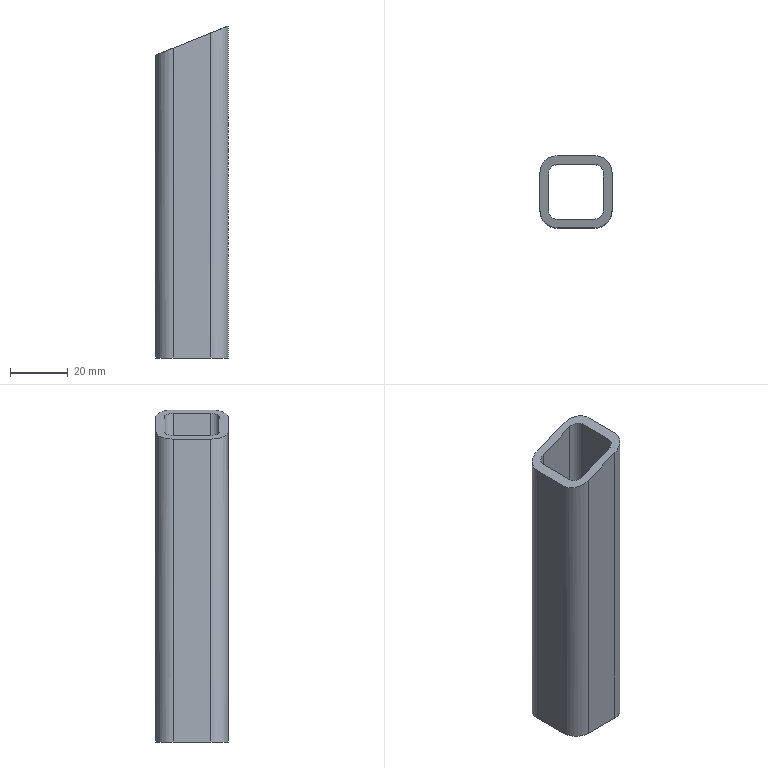Part | STEP file | ISO 10799-2 25x25x3 1784907954146 | 1 solid | 18 faces | box 25 x 25 x 115.036 mm | volume 26491 mm3 | plane 10 | cylinder 8 | commonest cylinder face diameters 6 x4 12 x4
STEP:
#1=CARTESIAN_POINT('',(12.5,6.5,115.036));
#2=VERTEX_POINT('',#1);
#3=CARTESIAN_POINT('',(12.5,-6.5,115.036));
#4=VERTEX_POINT('',#3);
#5=CARTESIAN_POINT('',(12.5,3.25,115.036));
#6=DIRECTION('',(0.,-1.,0.));
#7=VECTOR('',#6,10.);
#8=LINE('',#5,#7);
#9=EDGE_CURVE('',#2,#4,#8,.T.);
#10=ORIENTED_EDGE('',*,*,#9,.F.);
#11=CARTESIAN_POINT('',(6.5,12.5,112.619));
#12=VERTEX_POINT('',#11);
#13=CARTESIAN_POINT('',(6.5,6.5,112.619));
#14=DIRECTION('',(0.3737,0.,-0.9275));
#15=DIRECTION('',(-0.9275,0.,-0.3737));
#16=AXIS2_PLACEMENT_3D('',#13,#14,#15);
#17=ELLIPSE('',#16,6.469,6.);
#18=EDGE_CURVE('',#12,#2,#17,.T.);
#19=ORIENTED_EDGE('',*,*,#18,.F.);
#20=CARTESIAN_POINT('',(-6.5,12.5,107.381));
#21=VERTEX_POINT('',#20);
#22=CARTESIAN_POINT('',(-40.927,12.5,93.51));
#23=DIRECTION('',(0.9275,0.,0.3737));
#24=VECTOR('',#23,10.);
#25=LINE('',#22,#24);
#26=EDGE_CURVE('',#21,#12,#25,.T.);
#27=ORIENTED_EDGE('',*,*,#26,.F.);
#28=CARTESIAN_POINT('',(-12.5,6.5,104.964));
#29=VERTEX_POINT('',#28);
#30=CARTESIAN_POINT('',(-6.5,6.5,107.381));
#31=DIRECTION('',(0.3737,0.,-0.9275));
#32=DIRECTION('',(0.9275,0.,0.3737));
#33=AXIS2_PLACEMENT_3D('',#30,#31,#32);
#34=ELLIPSE('',#33,6.469,6.);
#35=EDGE_CURVE('',#29,#21,#34,.T.);
#36=ORIENTED_EDGE('',*,*,#35,.F.);
#37=CARTESIAN_POINT('',(-12.5,-6.5,104.964));
#38=VERTEX_POINT('',#37);
#39=CARTESIAN_POINT('',(-12.5,-3.25,104.964));
#40=DIRECTION('',(0.,1.,0.));
#41=VECTOR('',#40,10.);
#42=LINE('',#39,#41);
#43=EDGE_CURVE('',#38,#29,#42,.T.);
#44=ORIENTED_EDGE('',*,*,#43,.F.);
#45=CARTESIAN_POINT('',(-6.5,-12.5,107.381));
#46=VERTEX_POINT('',#45);
#47=CARTESIAN_POINT('',(-6.5,-6.5,107.381));
#48=DIRECTION('',(0.3737,0.,-0.9275));
#49=DIRECTION('',(0.9275,0.,0.3737));
#50=AXIS2_PLACEMENT_3D('',#47,#48,#49);
#51=ELLIPSE('',#50,6.469,6.);
#52=EDGE_CURVE('',#46,#38,#51,.T.);
#53=ORIENTED_EDGE('',*,*,#52,.F.);
#54=CARTESIAN_POINT('',(6.5,-12.5,112.619));
#55=VERTEX_POINT('',#54);
#56=CARTESIAN_POINT('',(-35.334,-12.5,95.763));
#57=DIRECTION('',(-0.9275,0.,-0.3737));
#58=VECTOR('',#57,10.);
#59=LINE('',#56,#58);
#60=EDGE_CURVE('',#55,#46,#59,.T.);
#61=ORIENTED_EDGE('',*,*,#60,.F.);
#62=CARTESIAN_POINT('',(6.5,-6.5,112.619));
#63=DIRECTION('',(0.3737,0.,-0.9275));
#64=DIRECTION('',(-0.9275,0.,-0.3737));
#65=AXIS2_PLACEMENT_3D('',#62,#63,#64);
#66=ELLIPSE('',#65,6.469,6.);
#67=EDGE_CURVE('',#4,#55,#66,.T.);
#68=ORIENTED_EDGE('',*,*,#67,.F.);
#69=EDGE_LOOP('',(#10,#19,#27,#36,#44,#53,#61,#68));
#70=FACE_OUTER_BOUND('',#69,.T.);
#71=CARTESIAN_POINT('',(-6.5,-9.5,107.381));
#72=VERTEX_POINT('',#71);
#73=CARTESIAN_POINT('',(6.5,-9.5,112.619));
#74=VERTEX_POINT('',#73);
#75=CARTESIAN_POINT('',(-35.334,-9.5,95.763));
#76=DIRECTION('',(0.9275,0.,0.3737));
#77=VECTOR('',#76,10.);
#78=LINE('',#75,#77);
#79=EDGE_CURVE('',#72,#74,#78,.T.);
#80=ORIENTED_EDGE('',*,*,#79,.F.);
#81=CARTESIAN_POINT('',(-9.5,-6.5,106.172));
#82=VERTEX_POINT('',#81);
#83=CARTESIAN_POINT('',(-6.5,-6.5,107.381));
#84=DIRECTION('',(-0.3737,0.,0.9275));
#85=DIRECTION('',(0.9275,0.,0.3737));
#86=AXIS2_PLACEMENT_3D('',#83,#84,#85);
#87=ELLIPSE('',#86,3.234,3.);
#88=EDGE_CURVE('',#82,#72,#87,.T.);
#89=ORIENTED_EDGE('',*,*,#88,.F.);
#90=CARTESIAN_POINT('',(-9.5,6.5,106.172));
#91=VERTEX_POINT('',#90);
#92=CARTESIAN_POINT('',(-9.5,-3.25,106.172));
#93=DIRECTION('',(0.,-1.,0.));
#94=VECTOR('',#93,10.);
#95=LINE('',#92,#94);
#96=EDGE_CURVE('',#91,#82,#95,.T.);
#97=ORIENTED_EDGE('',*,*,#96,.F.);
#98=CARTESIAN_POINT('',(-6.5,9.5,107.381));
#99=VERTEX_POINT('',#98);
#100=CARTESIAN_POINT('',(-6.5,6.5,107.381));
#101=DIRECTION('',(-0.3737,0.,0.9275));
#102=DIRECTION('',(0.9275,0.,0.3737));
#103=AXIS2_PLACEMENT_3D('',#100,#101,#102);
#104=ELLIPSE('',#103,3.234,3.);
#105=EDGE_CURVE('',#99,#91,#104,.T.);
#106=ORIENTED_EDGE('',*,*,#105,.F.);
#107=CARTESIAN_POINT('',(6.5,9.5,112.619));
#108=VERTEX_POINT('',#107);
#109=CARTESIAN_POINT('',(-40.927,9.5,93.51));
#110=DIRECTION('',(-0.9275,0.,-0.3737));
#111=VECTOR('',#110,10.);
#112=LINE('',#109,#111);
#113=EDGE_CURVE('',#108,#99,#112,.T.);
#114=ORIENTED_EDGE('',*,*,#113,.F.);
#115=CARTESIAN_POINT('',(9.5,6.5,113.828));
#116=VERTEX_POINT('',#115);
#117=CARTESIAN_POINT('',(6.5,6.5,112.619));
#118=DIRECTION('',(-0.3737,0.,0.9275));
#119=DIRECTION('',(-0.9275,0.,-0.3737));
#120=AXIS2_PLACEMENT_3D('',#117,#118,#119);
#121=ELLIPSE('',#120,3.234,3.);
#122=EDGE_CURVE('',#116,#108,#121,.T.);
#123=ORIENTED_EDGE('',*,*,#122,.F.);
#124=CARTESIAN_POINT('',(9.5,-6.5,113.828));
#125=VERTEX_POINT('',#124);
#126=CARTESIAN_POINT('',(9.5,3.25,113.828));
#127=DIRECTION('',(0.,1.,0.));
#128=VECTOR('',#127,10.);
#129=LINE('',#126,#128);
#130=EDGE_CURVE('',#125,#116,#129,.T.);
#131=ORIENTED_EDGE('',*,*,#130,.F.);
#132=CARTESIAN_POINT('',(6.5,-6.5,112.619));
#133=DIRECTION('',(-0.3737,0.,0.9275));
#134=DIRECTION('',(-0.9275,0.,-0.3737));
#135=AXIS2_PLACEMENT_3D('',#132,#133,#134);
#136=ELLIPSE('',#135,3.234,3.);
#137=EDGE_CURVE('',#74,#125,#136,.T.);
#138=ORIENTED_EDGE('',*,*,#137,.F.);
#139=EDGE_LOOP('',(#80,#89,#97,#106,#114,#123,#131,#138));
#140=FACE_BOUND('',#139,.T.);
#141=CARTESIAN_POINT('',(-38.131,0.,94.637));
#142=DIRECTION('',(0.3737,0.,-0.9275));
#143=DIRECTION('',(-0.9275,0.,-0.3737));
#144=AXIS2_PLACEMENT_3D('',#141,#142,#143);
#145=PLANE('',#144);
#146=ADVANCED_FACE('',(#70,#140),#145,.F.);
#147=ORIENTED_EDGE('',*,*,#113,.T.);
#148=CARTESIAN_POINT('',(-6.5,9.5,0.));
#149=VERTEX_POINT('',#148);
#150=CARTESIAN_POINT('',(-6.5,9.5,0.));
#151=DIRECTION('',(0.,0.,1.));
#152=VECTOR('',#151,10.);
#153=LINE('',#150,#152);
#154=EDGE_CURVE('',#149,#99,#153,.T.);
#155=ORIENTED_EDGE('',*,*,#154,.F.);
#156=CARTESIAN_POINT('',(6.5,9.5,0.));
#157=VERTEX_POINT('',#156);
#158=CARTESIAN_POINT('',(-3.25,9.5,0.));
#159=DIRECTION('',(-1.,0.,0.));
#160=VECTOR('',#159,10.);
#161=LINE('',#158,#160);
#162=EDGE_CURVE('',#157,#149,#161,.T.);
#163=ORIENTED_EDGE('',*,*,#162,.F.);
#164=CARTESIAN_POINT('',(6.5,9.5,0.));
#165=DIRECTION('',(0.,0.,1.));
#166=VECTOR('',#165,10.);
#167=LINE('',#164,#166);
#168=EDGE_CURVE('',#157,#108,#167,.T.);
#169=ORIENTED_EDGE('',*,*,#168,.T.);
#170=EDGE_LOOP('',(#147,#155,#163,#169));
#171=FACE_OUTER_BOUND('',#170,.T.);
#172=CARTESIAN_POINT('',(-6.5,9.5,0.));
#173=DIRECTION('',(0.,1.,0.));
#174=DIRECTION('',(0.,0.,1.));
#175=AXIS2_PLACEMENT_3D('',#172,#173,#174);
#176=PLANE('',#175);
#177=ADVANCED_FACE('',(#171),#176,.F.);
#178=ORIENTED_EDGE('',*,*,#105,.T.);
#179=CARTESIAN_POINT('',(-9.5,6.5,0.));
#180=VERTEX_POINT('',#179);
#181=CARTESIAN_POINT('',(-9.5,6.5,0.));
#182=DIRECTION('',(0.,0.,1.));
#183=VECTOR('',#182,10.);
#184=LINE('',#181,#183);
#185=EDGE_CURVE('',#180,#91,#184,.T.);
#186=ORIENTED_EDGE('',*,*,#185,.F.);
#187=CARTESIAN_POINT('',(-6.5,6.5,0.));
#188=DIRECTION('',(0.,0.,1.));
#189=DIRECTION('',(0.,-1.,0.));
#190=AXIS2_PLACEMENT_3D('',#187,#188,#189);
#191=CIRCLE('',#190,3.);
#192=EDGE_CURVE('',#149,#180,#191,.T.);
#193=ORIENTED_EDGE('',*,*,#192,.F.);
#194=ORIENTED_EDGE('',*,*,#154,.T.);
#195=EDGE_LOOP('',(#178,#186,#193,#194));
#196=FACE_OUTER_BOUND('',#195,.T.);
#197=CARTESIAN_POINT('',(-6.5,6.5,0.));
#198=DIRECTION('',(0.,0.,1.));
#199=DIRECTION('',(0.,-1.,0.));
#200=AXIS2_PLACEMENT_3D('',#197,#198,#199);
#201=CYLINDRICAL_SURFACE('',#200,3.);
#202=ADVANCED_FACE('',(#196),#201,.F.);
#203=ORIENTED_EDGE('',*,*,#96,.T.);
#204=CARTESIAN_POINT('',(-9.5,-6.5,0.));
#205=VERTEX_POINT('',#204);
#206=CARTESIAN_POINT('',(-9.5,-6.5,0.));
#207=DIRECTION('',(0.,0.,1.));
#208=VECTOR('',#207,10.);
#209=LINE('',#206,#208);
#210=EDGE_CURVE('',#205,#82,#209,.T.);
#211=ORIENTED_EDGE('',*,*,#210,.F.);
#212=CARTESIAN_POINT('',(-9.5,-3.25,0.));
#213=DIRECTION('',(0.,-1.,0.));
#214=VECTOR('',#213,10.);
#215=LINE('',#212,#214);
#216=EDGE_CURVE('',#180,#205,#215,.T.);
#217=ORIENTED_EDGE('',*,*,#216,.F.);
#218=ORIENTED_EDGE('',*,*,#185,.T.);
#219=EDGE_LOOP('',(#203,#211,#217,#218));
#220=FACE_OUTER_BOUND('',#219,.T.);
#221=CARTESIAN_POINT('',(-9.5,-6.5,0.));
#222=DIRECTION('',(-1.,0.,0.));
#223=DIRECTION('',(0.,0.,1.));
#224=AXIS2_PLACEMENT_3D('',#221,#222,#223);
#225=PLANE('',#224);
#226=ADVANCED_FACE('',(#220),#225,.F.);
#227=ORIENTED_EDGE('',*,*,#88,.T.);
#228=CARTESIAN_POINT('',(-6.5,-9.5,0.));
#229=VERTEX_POINT('',#228);
#230=CARTESIAN_POINT('',(-6.5,-9.5,0.));
#231=DIRECTION('',(0.,0.,1.));
#232=VECTOR('',#231,10.);
#233=LINE('',#230,#232);
#234=EDGE_CURVE('',#229,#72,#233,.T.);
#235=ORIENTED_EDGE('',*,*,#234,.F.);
#236=CARTESIAN_POINT('',(-6.5,-6.5,0.));
#237=DIRECTION('',(0.,0.,1.));
#238=DIRECTION('',(1.,0.,0.));
#239=AXIS2_PLACEMENT_3D('',#236,#237,#238);
#240=CIRCLE('',#239,3.);
#241=EDGE_CURVE('',#205,#229,#240,.T.);
#242=ORIENTED_EDGE('',*,*,#241,.F.);
#243=ORIENTED_EDGE('',*,*,#210,.T.);
#244=EDGE_LOOP('',(#227,#235,#242,#243));
#245=FACE_OUTER_BOUND('',#244,.T.);
#246=CARTESIAN_POINT('',(-6.5,-6.5,0.));
#247=DIRECTION('',(0.,0.,1.));
#248=DIRECTION('',(1.,0.,0.));
#249=AXIS2_PLACEMENT_3D('',#246,#247,#248);
#250=CYLINDRICAL_SURFACE('',#249,3.);
#251=ADVANCED_FACE('',(#245),#250,.F.);
#252=ORIENTED_EDGE('',*,*,#35,.T.);
#253=CARTESIAN_POINT('',(-6.5,12.5,0.));
#254=VERTEX_POINT('',#253);
#255=CARTESIAN_POINT('',(-6.5,12.5,0.));
#256=DIRECTION('',(0.,0.,1.));
#257=VECTOR('',#256,10.);
#258=LINE('',#255,#257);
#259=EDGE_CURVE('',#254,#21,#258,.T.);
#260=ORIENTED_EDGE('',*,*,#259,.F.);
#261=CARTESIAN_POINT('',(-12.5,6.5,0.));
#262=VERTEX_POINT('',#261);
#263=CARTESIAN_POINT('',(-6.5,6.5,0.));
#264=DIRECTION('',(0.,0.,-1.));
#265=DIRECTION('',(0.,-1.,0.));
#266=AXIS2_PLACEMENT_3D('',#263,#264,#265);
#267=CIRCLE('',#266,6.);
#268=EDGE_CURVE('',#262,#254,#267,.T.);
#269=ORIENTED_EDGE('',*,*,#268,.F.);
#270=CARTESIAN_POINT('',(-12.5,6.5,0.));
#271=DIRECTION('',(0.,0.,1.));
#272=VECTOR('',#271,10.);
#273=LINE('',#270,#272);
#274=EDGE_CURVE('',#262,#29,#273,.T.);
#275=ORIENTED_EDGE('',*,*,#274,.T.);
#276=EDGE_LOOP('',(#252,#260,#269,#275));
#277=FACE_OUTER_BOUND('',#276,.T.);
#278=CARTESIAN_POINT('',(-6.5,6.5,0.));
#279=DIRECTION('',(0.,0.,1.));
#280=DIRECTION('',(0.,-1.,0.));
#281=AXIS2_PLACEMENT_3D('',#278,#279,#280);
#282=CYLINDRICAL_SURFACE('',#281,6.);
#283=ADVANCED_FACE('',(#277),#282,.T.);
#284=ORIENTED_EDGE('',*,*,#26,.T.);
#285=CARTESIAN_POINT('',(6.5,12.5,0.));
#286=VERTEX_POINT('',#285);
#287=CARTESIAN_POINT('',(6.5,12.5,0.));
#288=DIRECTION('',(0.,0.,1.));
#289=VECTOR('',#288,10.);
#290=LINE('',#287,#289);
#291=EDGE_CURVE('',#286,#12,#290,.T.);
#292=ORIENTED_EDGE('',*,*,#291,.F.);
#293=CARTESIAN_POINT('',(-3.25,12.5,0.));
#294=DIRECTION('',(1.,0.,0.));
#295=VECTOR('',#294,10.);
#296=LINE('',#293,#295);
#297=EDGE_CURVE('',#254,#286,#296,.T.);
#298=ORIENTED_EDGE('',*,*,#297,.F.);
#299=ORIENTED_EDGE('',*,*,#259,.T.);
#300=EDGE_LOOP('',(#284,#292,#298,#299));
#301=FACE_OUTER_BOUND('',#300,.T.);
#302=CARTESIAN_POINT('',(-6.5,12.5,0.));
#303=DIRECTION('',(0.,1.,0.));
#304=DIRECTION('',(0.,0.,1.));
#305=AXIS2_PLACEMENT_3D('',#302,#303,#304);
#306=PLANE('',#305);
#307=ADVANCED_FACE('',(#301),#306,.T.);
#308=ORIENTED_EDGE('',*,*,#18,.T.);
#309=CARTESIAN_POINT('',(12.5,6.5,0.));
#310=VERTEX_POINT('',#309);
#311=CARTESIAN_POINT('',(12.5,6.5,0.));
#312=DIRECTION('',(0.,0.,1.));
#313=VECTOR('',#312,10.);
#314=LINE('',#311,#313);
#315=EDGE_CURVE('',#310,#2,#314,.T.);
#316=ORIENTED_EDGE('',*,*,#315,.F.);
#317=CARTESIAN_POINT('',(6.5,6.5,0.));
#318=DIRECTION('',(0.,0.,-1.));
#319=DIRECTION('',(-1.,0.,0.));
#320=AXIS2_PLACEMENT_3D('',#317,#318,#319);
#321=CIRCLE('',#320,6.);
#322=EDGE_CURVE('',#286,#310,#321,.T.);
#323=ORIENTED_EDGE('',*,*,#322,.F.);
#324=ORIENTED_EDGE('',*,*,#291,.T.);
#325=EDGE_LOOP('',(#308,#316,#323,#324));
#326=FACE_OUTER_BOUND('',#325,.T.);
#327=CARTESIAN_POINT('',(6.5,6.5,0.));
#328=DIRECTION('',(0.,0.,1.));
#329=DIRECTION('',(-1.,0.,0.));
#330=AXIS2_PLACEMENT_3D('',#327,#328,#329);
#331=CYLINDRICAL_SURFACE('',#330,6.);
#332=ADVANCED_FACE('',(#326),#331,.T.);
#333=ORIENTED_EDGE('',*,*,#79,.T.);
#334=CARTESIAN_POINT('',(6.5,-9.5,0.));
#335=VERTEX_POINT('',#334);
#336=CARTESIAN_POINT('',(6.5,-9.5,0.));
#337=DIRECTION('',(0.,0.,1.));
#338=VECTOR('',#337,10.);
#339=LINE('',#336,#338);
#340=EDGE_CURVE('',#335,#74,#339,.T.);
#341=ORIENTED_EDGE('',*,*,#340,.F.);
#342=CARTESIAN_POINT('',(3.25,-9.5,0.));
#343=DIRECTION('',(1.,0.,0.));
#344=VECTOR('',#343,10.);
#345=LINE('',#342,#344);
#346=EDGE_CURVE('',#229,#335,#345,.T.);
#347=ORIENTED_EDGE('',*,*,#346,.F.);
#348=ORIENTED_EDGE('',*,*,#234,.T.);
#349=EDGE_LOOP('',(#333,#341,#347,#348));
#350=FACE_OUTER_BOUND('',#349,.T.);
#351=CARTESIAN_POINT('',(6.5,-9.5,0.));
#352=DIRECTION('',(0.,-1.,0.));
#353=DIRECTION('',(0.,0.,-1.));
#354=AXIS2_PLACEMENT_3D('',#351,#352,#353);
#355=PLANE('',#354);
#356=ADVANCED_FACE('',(#350),#355,.F.);
#357=ORIENTED_EDGE('',*,*,#137,.T.);
#358=CARTESIAN_POINT('',(9.5,-6.5,0.));
#359=VERTEX_POINT('',#358);
#360=CARTESIAN_POINT('',(9.5,-6.5,0.));
#361=DIRECTION('',(0.,0.,1.));
#362=VECTOR('',#361,10.);
#363=LINE('',#360,#362);
#364=EDGE_CURVE('',#359,#125,#363,.T.);
#365=ORIENTED_EDGE('',*,*,#364,.F.);
#366=CARTESIAN_POINT('',(6.5,-6.5,0.));
#367=DIRECTION('',(0.,0.,1.));
#368=DIRECTION('',(0.,1.,0.));
#369=AXIS2_PLACEMENT_3D('',#366,#367,#368);
#370=CIRCLE('',#369,3.);
#371=EDGE_CURVE('',#335,#359,#370,.T.);
#372=ORIENTED_EDGE('',*,*,#371,.F.);
#373=ORIENTED_EDGE('',*,*,#340,.T.);
#374=EDGE_LOOP('',(#357,#365,#372,#373));
#375=FACE_OUTER_BOUND('',#374,.T.);
#376=CARTESIAN_POINT('',(6.5,-6.5,0.));
#377=DIRECTION('',(0.,0.,1.));
#378=DIRECTION('',(0.,1.,0.));
#379=AXIS2_PLACEMENT_3D('',#376,#377,#378);
#380=CYLINDRICAL_SURFACE('',#379,3.);
#381=ADVANCED_FACE('',(#375),#380,.F.);
#382=ORIENTED_EDGE('',*,*,#130,.T.);
#383=CARTESIAN_POINT('',(9.5,6.5,0.));
#384=VERTEX_POINT('',#383);
#385=CARTESIAN_POINT('',(9.5,6.5,0.));
#386=DIRECTION('',(0.,0.,1.));
#387=VECTOR('',#386,10.);
#388=LINE('',#385,#387);
#389=EDGE_CURVE('',#384,#116,#388,.T.);
#390=ORIENTED_EDGE('',*,*,#389,.F.);
#391=CARTESIAN_POINT('',(9.5,3.25,0.));
#392=DIRECTION('',(0.,1.,0.));
#393=VECTOR('',#392,10.);
#394=LINE('',#391,#393);
#395=EDGE_CURVE('',#359,#384,#394,.T.);
#396=ORIENTED_EDGE('',*,*,#395,.F.);
#397=ORIENTED_EDGE('',*,*,#364,.T.);
#398=EDGE_LOOP('',(#382,#390,#396,#397));
#399=FACE_OUTER_BOUND('',#398,.T.);
#400=CARTESIAN_POINT('',(9.5,6.5,0.));
#401=DIRECTION('',(1.,0.,0.));
#402=DIRECTION('',(0.,0.,-1.));
#403=AXIS2_PLACEMENT_3D('',#400,#401,#402);
#404=PLANE('',#403);
#405=ADVANCED_FACE('',(#399),#404,.F.);
#406=ORIENTED_EDGE('',*,*,#122,.T.);
#407=ORIENTED_EDGE('',*,*,#168,.F.);
#408=CARTESIAN_POINT('',(6.5,6.5,0.));
#409=DIRECTION('',(0.,0.,1.));
#410=DIRECTION('',(-1.,0.,0.));
#411=AXIS2_PLACEMENT_3D('',#408,#409,#410);
#412=CIRCLE('',#411,3.);
#413=EDGE_CURVE('',#384,#157,#412,.T.);
#414=ORIENTED_EDGE('',*,*,#413,.F.);
#415=ORIENTED_EDGE('',*,*,#389,.T.);
#416=EDGE_LOOP('',(#406,#407,#414,#415));
#417=FACE_OUTER_BOUND('',#416,.T.);
#418=CARTESIAN_POINT('',(6.5,6.5,0.));
#419=DIRECTION('',(0.,0.,1.));
#420=DIRECTION('',(-1.,0.,0.));
#421=AXIS2_PLACEMENT_3D('',#418,#419,#420);
#422=CYLINDRICAL_SURFACE('',#421,3.);
#423=ADVANCED_FACE('',(#417),#422,.F.);
#424=ORIENTED_EDGE('',*,*,#9,.T.);
#425=CARTESIAN_POINT('',(12.5,-6.5,0.));
#426=VERTEX_POINT('',#425);
#427=CARTESIAN_POINT('',(12.5,-6.5,0.));
#428=DIRECTION('',(0.,0.,1.));
#429=VECTOR('',#428,10.);
#430=LINE('',#427,#429);
#431=EDGE_CURVE('',#426,#4,#430,.T.);
#432=ORIENTED_EDGE('',*,*,#431,.F.);
#433=CARTESIAN_POINT('',(12.5,3.25,0.));
#434=DIRECTION('',(0.,-1.,0.));
#435=VECTOR('',#434,10.);
#436=LINE('',#433,#435);
#437=EDGE_CURVE('',#310,#426,#436,.T.);
#438=ORIENTED_EDGE('',*,*,#437,.F.);
#439=ORIENTED_EDGE('',*,*,#315,.T.);
#440=EDGE_LOOP('',(#424,#432,#438,#439));
#441=FACE_OUTER_BOUND('',#440,.T.);
#442=CARTESIAN_POINT('',(12.5,6.5,0.));
#443=DIRECTION('',(1.,0.,0.));
#444=DIRECTION('',(0.,0.,-1.));
#445=AXIS2_PLACEMENT_3D('',#442,#443,#444);
#446=PLANE('',#445);
#447=ADVANCED_FACE('',(#441),#446,.T.);
#448=ORIENTED_EDGE('',*,*,#67,.T.);
#449=CARTESIAN_POINT('',(6.5,-12.5,0.));
#450=VERTEX_POINT('',#449);
#451=CARTESIAN_POINT('',(6.5,-12.5,0.));
#452=DIRECTION('',(0.,0.,1.));
#453=VECTOR('',#452,10.);
#454=LINE('',#451,#453);
#455=EDGE_CURVE('',#450,#55,#454,.T.);
#456=ORIENTED_EDGE('',*,*,#455,.F.);
#457=CARTESIAN_POINT('',(6.5,-6.5,0.));
#458=DIRECTION('',(0.,0.,-1.));
#459=DIRECTION('',(0.,1.,0.));
#460=AXIS2_PLACEMENT_3D('',#457,#458,#459);
#461=CIRCLE('',#460,6.);
#462=EDGE_CURVE('',#426,#450,#461,.T.);
#463=ORIENTED_EDGE('',*,*,#462,.F.);
#464=ORIENTED_EDGE('',*,*,#431,.T.);
#465=EDGE_LOOP('',(#448,#456,#463,#464));
#466=FACE_OUTER_BOUND('',#465,.T.);
#467=CARTESIAN_POINT('',(6.5,-6.5,0.));
#468=DIRECTION('',(0.,0.,1.));
#469=DIRECTION('',(0.,1.,0.));
#470=AXIS2_PLACEMENT_3D('',#467,#468,#469);
#471=CYLINDRICAL_SURFACE('',#470,6.);
#472=ADVANCED_FACE('',(#466),#471,.T.);
#473=ORIENTED_EDGE('',*,*,#60,.T.);
#474=CARTESIAN_POINT('',(-6.5,-12.5,0.));
#475=VERTEX_POINT('',#474);
#476=CARTESIAN_POINT('',(-6.5,-12.5,0.));
#477=DIRECTION('',(0.,0.,1.));
#478=VECTOR('',#477,10.);
#479=LINE('',#476,#478);
#480=EDGE_CURVE('',#475,#46,#479,.T.);
#481=ORIENTED_EDGE('',*,*,#480,.F.);
#482=CARTESIAN_POINT('',(3.25,-12.5,0.));
#483=DIRECTION('',(-1.,0.,0.));
#484=VECTOR('',#483,10.);
#485=LINE('',#482,#484);
#486=EDGE_CURVE('',#450,#475,#485,.T.);
#487=ORIENTED_EDGE('',*,*,#486,.F.);
#488=ORIENTED_EDGE('',*,*,#455,.T.);
#489=EDGE_LOOP('',(#473,#481,#487,#488));
#490=FACE_OUTER_BOUND('',#489,.T.);
#491=CARTESIAN_POINT('',(6.5,-12.5,0.));
#492=DIRECTION('',(0.,-1.,0.));
#493=DIRECTION('',(0.,0.,-1.));
#494=AXIS2_PLACEMENT_3D('',#491,#492,#493);
#495=PLANE('',#494);
#496=ADVANCED_FACE('',(#490),#495,.T.);
#497=ORIENTED_EDGE('',*,*,#52,.T.);
#498=CARTESIAN_POINT('',(-12.5,-6.5,0.));
#499=VERTEX_POINT('',#498);
#500=CARTESIAN_POINT('',(-12.5,-6.5,0.));
#501=DIRECTION('',(0.,0.,1.));
#502=VECTOR('',#501,10.);
#503=LINE('',#500,#502);
#504=EDGE_CURVE('',#499,#38,#503,.T.);
#505=ORIENTED_EDGE('',*,*,#504,.F.);
#506=CARTESIAN_POINT('',(-6.5,-6.5,0.));
#507=DIRECTION('',(0.,0.,-1.));
#508=DIRECTION('',(1.,0.,0.));
#509=AXIS2_PLACEMENT_3D('',#506,#507,#508);
#510=CIRCLE('',#509,6.);
#511=EDGE_CURVE('',#475,#499,#510,.T.);
#512=ORIENTED_EDGE('',*,*,#511,.F.);
#513=ORIENTED_EDGE('',*,*,#480,.T.);
#514=EDGE_LOOP('',(#497,#505,#512,#513));
#515=FACE_OUTER_BOUND('',#514,.T.);
#516=CARTESIAN_POINT('',(-6.5,-6.5,0.));
#517=DIRECTION('',(0.,0.,1.));
#518=DIRECTION('',(1.,0.,0.));
#519=AXIS2_PLACEMENT_3D('',#516,#517,#518);
#520=CYLINDRICAL_SURFACE('',#519,6.);
#521=ADVANCED_FACE('',(#515),#520,.T.);
#522=ORIENTED_EDGE('',*,*,#43,.T.);
#523=ORIENTED_EDGE('',*,*,#274,.F.);
#524=CARTESIAN_POINT('',(-12.5,-3.25,0.));
#525=DIRECTION('',(0.,1.,0.));
#526=VECTOR('',#525,10.);
#527=LINE('',#524,#526);
#528=EDGE_CURVE('',#499,#262,#527,.T.);
#529=ORIENTED_EDGE('',*,*,#528,.F.);
#530=ORIENTED_EDGE('',*,*,#504,.T.);
#531=EDGE_LOOP('',(#522,#523,#529,#530));
#532=FACE_OUTER_BOUND('',#531,.T.);
#533=CARTESIAN_POINT('',(-12.5,-6.5,0.));
#534=DIRECTION('',(-1.,0.,0.));
#535=DIRECTION('',(0.,0.,1.));
#536=AXIS2_PLACEMENT_3D('',#533,#534,#535);
#537=PLANE('',#536);
#538=ADVANCED_FACE('',(#532),#537,.T.);
#539=ORIENTED_EDGE('',*,*,#528,.T.);
#540=ORIENTED_EDGE('',*,*,#268,.T.);
#541=ORIENTED_EDGE('',*,*,#297,.T.);
#542=ORIENTED_EDGE('',*,*,#322,.T.);
#543=ORIENTED_EDGE('',*,*,#437,.T.);
#544=ORIENTED_EDGE('',*,*,#462,.T.);
#545=ORIENTED_EDGE('',*,*,#486,.T.);
#546=ORIENTED_EDGE('',*,*,#511,.T.);
#547=EDGE_LOOP('',(#539,#540,#541,#542,#543,#544,#545,#546));
#548=FACE_OUTER_BOUND('',#547,.T.);
#549=ORIENTED_EDGE('',*,*,#162,.T.);
#550=ORIENTED_EDGE('',*,*,#192,.T.);
#551=ORIENTED_EDGE('',*,*,#216,.T.);
#552=ORIENTED_EDGE('',*,*,#241,.T.);
#553=ORIENTED_EDGE('',*,*,#346,.T.);
#554=ORIENTED_EDGE('',*,*,#371,.T.);
#555=ORIENTED_EDGE('',*,*,#395,.T.);
#556=ORIENTED_EDGE('',*,*,#413,.T.);
#557=EDGE_LOOP('',(#549,#550,#551,#552,#553,#554,#555,#556));
#558=FACE_BOUND('',#557,.T.);
#559=CARTESIAN_POINT('',(0.,0.,0.));
#560=DIRECTION('',(0.,0.,1.));
#561=DIRECTION('',(1.,0.,0.));
#562=AXIS2_PLACEMENT_3D('',#559,#560,#561);
#563=PLANE('',#562);
#564=ADVANCED_FACE('',(#548,#558),#563,.F.);
#565=CLOSED_SHELL('',(#146,#177,#202,#226,#251,#283,#307,#332,#356,#381,#405,#423,#447,#472,#496,#521,#538,#564));
#566=MANIFOLD_SOLID_BREP('',#565);
#567=(LENGTH_UNIT()NAMED_UNIT(*)SI_UNIT(.MILLI.,.METRE.));
#568=UNCERTAINTY_MEASURE_WITH_UNIT(LENGTH_MEASURE(0.01),#567,'','');
#569=(NAMED_UNIT(*)PLANE_ANGLE_UNIT()SI_UNIT($,.RADIAN.));
#570=(NAMED_UNIT(*)SI_UNIT($,.STERADIAN.)SOLID_ANGLE_UNIT());
#571=(GEOMETRIC_REPRESENTATION_CONTEXT(3)GLOBAL_UNCERTAINTY_ASSIGNED_CONTEXT((#568))GLOBAL_UNIT_ASSIGNED_CONTEXT((#567,#569,#570))REPRESENTATION_CONTEXT('',''));
#572=ADVANCED_BREP_SHAPE_REPRESENTATION('',(#566),#571);